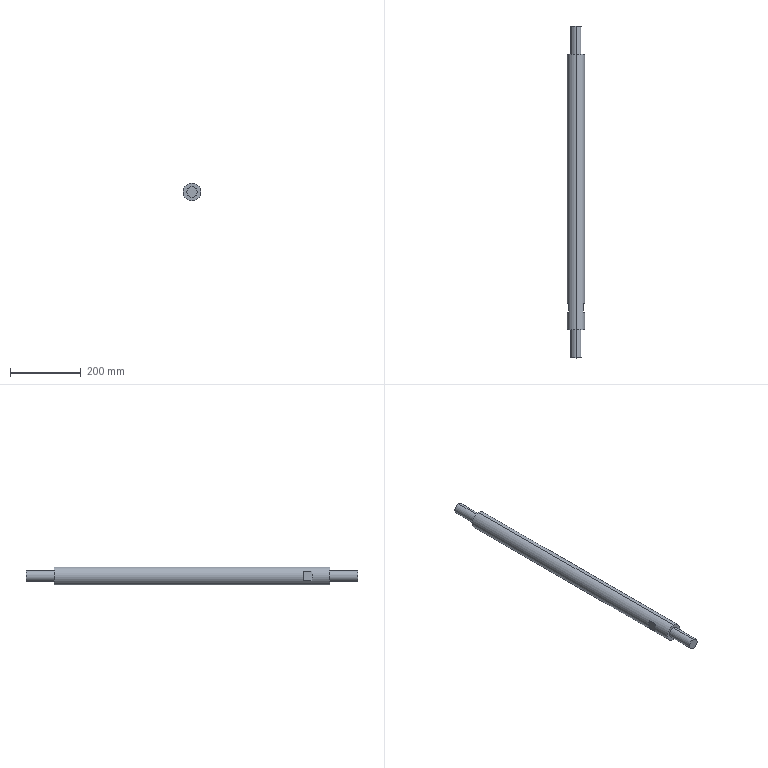Part | STEP file | 1 solid | 16 faces | box 50 x 940 x 50 mm | volume 1640944 mm3 | plane 10 | cylinder 6 | commonest cylinder face diameters 30 x4 50 x2
STEP:
#1=CARTESIAN_POINT('',(0.,0.,0.));
#2=DIRECTION('',(0.,0.,1.));
#3=DIRECTION('',(1.,0.,0.));
#4=AXIS2_PLACEMENT_3D('',#1,#2,#3);
#5=CARTESIAN_POINT('',(0.,940.,-15.));
#6=VERTEX_POINT('',#5);
#7=CARTESIAN_POINT('',(0.,940.,15.));
#8=VERTEX_POINT('',#7);
#9=CARTESIAN_POINT('',(0.,940.,0.));
#10=DIRECTION('',(0.,-1.,0.));
#11=DIRECTION('',(0.,0.,-1.));
#12=AXIS2_PLACEMENT_3D('',#9,#10,#11);
#13=CIRCLE('',#12,15.);
#14=CARTESIAN_POINT('',(0.,0.,0.));
#15=DIRECTION('',(0.,-1.,0.));
#16=DIRECTION('',(0.,0.,-1.));
#17=AXIS2_PLACEMENT_3D('',#14,#15,#16);
#18=CYLINDRICAL_SURFACE('',#17,15.);
#19=CARTESIAN_POINT('',(0.,-940.));
#20=DIRECTION('',(1.,0.));
#21=VECTOR('',#20,1.);
#22=LINE('',#19,#21);
#23=(GEOMETRIC_REPRESENTATION_CONTEXT(2)PARAMETRIC_REPRESENTATION_CONTEXT()REPRESENTATION_CONTEXT('',''));
#24=DEFINITIONAL_REPRESENTATION('',(#22),#23);
#25=PCURVE('',#18,#24);
#26=CARTESIAN_POINT('',(15.,940.,0.));
#27=DIRECTION('',(0.,1.,0.));
#28=DIRECTION('',(0.,0.,1.));
#29=AXIS2_PLACEMENT_3D('',#26,#27,#28);
#30=PLANE('',#29);
#31=CARTESIAN_POINT('',(-15.,-15.));
#32=CARTESIAN_POINT('',(-15.,10.981));
#33=CARTESIAN_POINT('',(7.5,-2.01));
#34=CARTESIAN_POINT('',(30.,-15.));
#35=CARTESIAN_POINT('',(7.5,-27.99));
#36=CARTESIAN_POINT('',(-15.,-40.981));
#37=CARTESIAN_POINT('',(-15.,-15.));
#38=(BOUNDED_CURVE()B_SPLINE_CURVE(2,(#31,#32,#33,#34,#35,#36,#37),.UNSPECIFIED.,.T.,.F.)B_SPLINE_CURVE_WITH_KNOTS((1,2,2,2,2,1),(-2.094,0.,2.094,4.189,6.283,8.378),.UNSPECIFIED.)CURVE()GEOMETRIC_REPRESENTATION_ITEM()RATIONAL_B_SPLINE_CURVE((1.,0.5,1.,0.5,1.,0.5,1.))REPRESENTATION_ITEM(''));
#39=(GEOMETRIC_REPRESENTATION_CONTEXT(2)PARAMETRIC_REPRESENTATION_CONTEXT()REPRESENTATION_CONTEXT('',''));
#40=DEFINITIONAL_REPRESENTATION('',(#38),#39);
#41=PCURVE('',#30,#40);
#42=SURFACE_CURVE('',#13,(#25,#41),.PCURVE_S1.);
#43=EDGE_CURVE('',#6,#8,#42,.T.);
#44=ORIENTED_EDGE('',*,*,#43,.T.);
#45=CARTESIAN_POINT('',(0.,860.,15.));
#46=VERTEX_POINT('',#45);
#47=CARTESIAN_POINT('',(0.,0.,15.));
#48=DIRECTION('',(0.,-1.,0.));
#49=VECTOR('',#48,1.);
#50=LINE('',#47,#49);
#51=CARTESIAN_POINT('',(3.142,0.));
#52=DIRECTION('',(0.,1.));
#53=VECTOR('',#52,1.);
#54=LINE('',#51,#53);
#55=(GEOMETRIC_REPRESENTATION_CONTEXT(2)PARAMETRIC_REPRESENTATION_CONTEXT()REPRESENTATION_CONTEXT('',''));
#56=DEFINITIONAL_REPRESENTATION('',(#54),#55);
#57=PCURVE('',#18,#56);
#58=CARTESIAN_POINT('',(0.,0.,0.));
#59=DIRECTION('',(0.,-1.,0.));
#60=DIRECTION('',(0.,0.,-1.));
#61=AXIS2_PLACEMENT_3D('',#58,#59,#60);
#62=CYLINDRICAL_SURFACE('',#61,15.);
#63=CARTESIAN_POINT('',(3.142,0.));
#64=DIRECTION('',(0.,1.));
#65=VECTOR('',#64,1.);
#66=LINE('',#63,#65);
#67=(GEOMETRIC_REPRESENTATION_CONTEXT(2)PARAMETRIC_REPRESENTATION_CONTEXT()REPRESENTATION_CONTEXT('',''));
#68=DEFINITIONAL_REPRESENTATION('',(#66),#67);
#69=PCURVE('',#62,#68);
#70=SURFACE_CURVE('',#50,(#57,#69),.PCURVE_S1.);
#71=EDGE_CURVE('',#8,#46,#70,.T.);
#72=ORIENTED_EDGE('',*,*,#71,.T.);
#73=CARTESIAN_POINT('',(0.,860.,-15.));
#74=VERTEX_POINT('',#73);
#75=CARTESIAN_POINT('',(0.,860.,0.));
#76=DIRECTION('',(0.,-1.,0.));
#77=DIRECTION('',(0.,0.,-1.));
#78=AXIS2_PLACEMENT_3D('',#75,#76,#77);
#79=CIRCLE('',#78,15.);
#80=CARTESIAN_POINT('',(0.,-860.));
#81=DIRECTION('',(1.,0.));
#82=VECTOR('',#81,1.);
#83=LINE('',#80,#82);
#84=(GEOMETRIC_REPRESENTATION_CONTEXT(2)PARAMETRIC_REPRESENTATION_CONTEXT()REPRESENTATION_CONTEXT('',''));
#85=DEFINITIONAL_REPRESENTATION('',(#83),#84);
#86=PCURVE('',#18,#85);
#87=CARTESIAN_POINT('',(25.,860.,0.));
#88=DIRECTION('',(0.,1.,0.));
#89=DIRECTION('',(0.,0.,1.));
#90=AXIS2_PLACEMENT_3D('',#87,#88,#89);
#91=PLANE('',#90);
#92=CARTESIAN_POINT('',(-15.,-25.));
#93=CARTESIAN_POINT('',(-15.,0.9808));
#94=CARTESIAN_POINT('',(7.5,-12.01));
#95=CARTESIAN_POINT('',(30.,-25.));
#96=CARTESIAN_POINT('',(7.5,-37.99));
#97=CARTESIAN_POINT('',(-15.,-50.981));
#98=CARTESIAN_POINT('',(-15.,-25.));
#99=(BOUNDED_CURVE()B_SPLINE_CURVE(2,(#92,#93,#94,#95,#96,#97,#98),.UNSPECIFIED.,.T.,.F.)B_SPLINE_CURVE_WITH_KNOTS((1,2,2,2,2,1),(-2.094,0.,2.094,4.189,6.283,8.378),.UNSPECIFIED.)CURVE()GEOMETRIC_REPRESENTATION_ITEM()RATIONAL_B_SPLINE_CURVE((1.,0.5,1.,0.5,1.,0.5,1.))REPRESENTATION_ITEM(''));
#100=(GEOMETRIC_REPRESENTATION_CONTEXT(2)PARAMETRIC_REPRESENTATION_CONTEXT()REPRESENTATION_CONTEXT('',''));
#101=DEFINITIONAL_REPRESENTATION('',(#99),#100);
#102=PCURVE('',#91,#101);
#103=SURFACE_CURVE('',#79,(#86,#102),.PCURVE_S1.);
#104=EDGE_CURVE('',#74,#46,#103,.T.);
#105=ORIENTED_EDGE('',*,*,#104,.F.);
#106=CARTESIAN_POINT('',(0.,0.,-15.));
#107=DIRECTION('',(0.,-1.,0.));
#108=VECTOR('',#107,1.);
#109=LINE('',#106,#108);
#110=CARTESIAN_POINT('',(0.,0.));
#111=DIRECTION('',(0.,1.));
#112=VECTOR('',#111,1.);
#113=LINE('',#110,#112);
#114=(GEOMETRIC_REPRESENTATION_CONTEXT(2)PARAMETRIC_REPRESENTATION_CONTEXT()REPRESENTATION_CONTEXT('',''));
#115=DEFINITIONAL_REPRESENTATION('',(#113),#114);
#116=PCURVE('',#18,#115);
#117=CARTESIAN_POINT('',(6.283,0.));
#118=DIRECTION('',(0.,1.));
#119=VECTOR('',#118,1.);
#120=LINE('',#117,#119);
#121=(GEOMETRIC_REPRESENTATION_CONTEXT(2)PARAMETRIC_REPRESENTATION_CONTEXT()REPRESENTATION_CONTEXT('',''));
#122=DEFINITIONAL_REPRESENTATION('',(#120),#121);
#123=PCURVE('',#62,#122);
#124=SURFACE_CURVE('',#109,(#116,#123),.PCURVE_S1.);
#125=EDGE_CURVE('',#6,#74,#124,.T.);
#126=ORIENTED_EDGE('',*,*,#125,.F.);
#127=EDGE_LOOP('',(#44,#72,#105,#126));
#128=FACE_BOUND('',#127,.T.);
#129=ADVANCED_FACE('',(#128),#18,.T.);
#130=CARTESIAN_POINT('',(21.,130.,-13.565));
#131=VERTEX_POINT('',#130);
#132=CARTESIAN_POINT('',(21.,155.,-13.565));
#133=VERTEX_POINT('',#132);
#134=CARTESIAN_POINT('',(21.,0.,-13.565));
#135=DIRECTION('',(0.,1.,0.));
#136=VECTOR('',#135,1.);
#137=LINE('',#134,#136);
#138=CARTESIAN_POINT('',(0.,0.,0.));
#139=DIRECTION('',(0.,-1.,0.));
#140=DIRECTION('',(0.,0.,-1.));
#141=AXIS2_PLACEMENT_3D('',#138,#139,#140);
#142=CYLINDRICAL_SURFACE('',#141,25.);
#143=CARTESIAN_POINT('',(0.9973,0.));
#144=DIRECTION('',(0.,-1.));
#145=VECTOR('',#144,1.);
#146=LINE('',#143,#145);
#147=(GEOMETRIC_REPRESENTATION_CONTEXT(2)PARAMETRIC_REPRESENTATION_CONTEXT()REPRESENTATION_CONTEXT('',''));
#148=DEFINITIONAL_REPRESENTATION('',(#146),#147);
#149=PCURVE('',#142,#148);
#150=CARTESIAN_POINT('',(21.,155.,-30.));
#151=DIRECTION('',(-1.,0.,0.));
#152=DIRECTION('',(0.,0.,1.));
#153=AXIS2_PLACEMENT_3D('',#150,#151,#152);
#154=PLANE('',#153);
#155=CARTESIAN_POINT('',(16.435,-155.));
#156=DIRECTION('',(0.,1.));
#157=VECTOR('',#156,1.);
#158=LINE('',#155,#157);
#159=(GEOMETRIC_REPRESENTATION_CONTEXT(2)PARAMETRIC_REPRESENTATION_CONTEXT()REPRESENTATION_CONTEXT('',''));
#160=DEFINITIONAL_REPRESENTATION('',(#158),#159);
#161=PCURVE('',#154,#160);
#162=SURFACE_CURVE('',#137,(#149,#161),.PCURVE_S1.);
#163=EDGE_CURVE('',#131,#133,#162,.T.);
#164=ORIENTED_EDGE('',*,*,#163,.F.);
#165=CARTESIAN_POINT('',(21.,130.,13.565));
#166=VERTEX_POINT('',#165);
#167=CARTESIAN_POINT('',(0.,130.,0.));
#168=DIRECTION('',(0.,1.,0.));
#169=DIRECTION('',(0.,0.,-1.));
#170=AXIS2_PLACEMENT_3D('',#167,#168,#169);
#171=CIRCLE('',#170,25.);
#172=CARTESIAN_POINT('',(6.283,-130.));
#173=DIRECTION('',(-1.,0.));
#174=VECTOR('',#173,1.);
#175=LINE('',#172,#174);
#176=(GEOMETRIC_REPRESENTATION_CONTEXT(2)PARAMETRIC_REPRESENTATION_CONTEXT()REPRESENTATION_CONTEXT('',''));
#177=DEFINITIONAL_REPRESENTATION('',(#175),#176);
#178=PCURVE('',#142,#177);
#179=CARTESIAN_POINT('',(65.117,130.,-30.));
#180=DIRECTION('',(0.,-1.,0.));
#181=DIRECTION('',(0.,0.,-1.));
#182=AXIS2_PLACEMENT_3D('',#179,#180,#181);
#183=PLANE('',#182);
#184=CARTESIAN_POINT('',(-5.,-65.117));
#185=CARTESIAN_POINT('',(-5.,-108.419));
#186=CARTESIAN_POINT('',(-42.5,-86.768));
#187=CARTESIAN_POINT('',(-80.,-65.117));
#188=CARTESIAN_POINT('',(-42.5,-43.467));
#189=CARTESIAN_POINT('',(-5.,-21.816));
#190=CARTESIAN_POINT('',(-5.,-65.117));
#191=(BOUNDED_CURVE()B_SPLINE_CURVE(2,(#184,#185,#186,#187,#188,#189,#190),.UNSPECIFIED.,.T.,.F.)B_SPLINE_CURVE_WITH_KNOTS((1,2,2,2,2,1),(-2.094,0.,2.094,4.189,6.283,8.378),.UNSPECIFIED.)CURVE()GEOMETRIC_REPRESENTATION_ITEM()RATIONAL_B_SPLINE_CURVE((1.,0.5,1.,0.5,1.,0.5,1.))REPRESENTATION_ITEM(''));
#192=(GEOMETRIC_REPRESENTATION_CONTEXT(2)PARAMETRIC_REPRESENTATION_CONTEXT()REPRESENTATION_CONTEXT('',''));
#193=DEFINITIONAL_REPRESENTATION('',(#191),#192);
#194=PCURVE('',#183,#193);
#195=SURFACE_CURVE('',#171,(#178,#194),.PCURVE_S1.);
#196=EDGE_CURVE('',#166,#131,#195,.T.);
#197=ORIENTED_EDGE('',*,*,#196,.F.);
#198=CARTESIAN_POINT('',(21.,155.,13.565));
#199=VERTEX_POINT('',#198);
#200=CARTESIAN_POINT('',(21.,0.,13.565));
#201=DIRECTION('',(0.,-1.,0.));
#202=VECTOR('',#201,1.);
#203=LINE('',#200,#202);
#204=CARTESIAN_POINT('',(2.144,0.));
#205=DIRECTION('',(0.,1.));
#206=VECTOR('',#205,1.);
#207=LINE('',#204,#206);
#208=(GEOMETRIC_REPRESENTATION_CONTEXT(2)PARAMETRIC_REPRESENTATION_CONTEXT()REPRESENTATION_CONTEXT('',''));
#209=DEFINITIONAL_REPRESENTATION('',(#207),#208);
#210=PCURVE('',#142,#209);
#211=CARTESIAN_POINT('',(43.565,-155.));
#212=DIRECTION('',(0.,-1.));
#213=VECTOR('',#212,1.);
#214=LINE('',#211,#213);
#215=(GEOMETRIC_REPRESENTATION_CONTEXT(2)PARAMETRIC_REPRESENTATION_CONTEXT()REPRESENTATION_CONTEXT('',''));
#216=DEFINITIONAL_REPRESENTATION('',(#214),#215);
#217=PCURVE('',#154,#216);
#218=SURFACE_CURVE('',#203,(#210,#217),.PCURVE_S1.);
#219=EDGE_CURVE('',#199,#166,#218,.T.);
#220=ORIENTED_EDGE('',*,*,#219,.F.);
#221=CARTESIAN_POINT('',(0.,155.,0.));
#222=DIRECTION('',(0.,-1.,0.));
#223=DIRECTION('',(0.,0.,1.));
#224=AXIS2_PLACEMENT_3D('',#221,#222,#223);
#225=CIRCLE('',#224,25.);
#226=CARTESIAN_POINT('',(-3.142,-155.));
#227=DIRECTION('',(1.,0.));
#228=VECTOR('',#227,1.);
#229=LINE('',#226,#228);
#230=(GEOMETRIC_REPRESENTATION_CONTEXT(2)PARAMETRIC_REPRESENTATION_CONTEXT()REPRESENTATION_CONTEXT('',''));
#231=DEFINITIONAL_REPRESENTATION('',(#229),#230);
#232=PCURVE('',#142,#231);
#233=CARTESIAN_POINT('',(65.117,155.,-30.));
#234=DIRECTION('',(0.,1.,0.));
#235=DIRECTION('',(0.,0.,1.));
#236=AXIS2_PLACEMENT_3D('',#233,#234,#235);
#237=PLANE('',#236);
#238=CARTESIAN_POINT('',(55.,-65.117));
#239=CARTESIAN_POINT('',(55.,-108.419));
#240=CARTESIAN_POINT('',(17.5,-86.768));
#241=CARTESIAN_POINT('',(-20.,-65.117));
#242=CARTESIAN_POINT('',(17.5,-43.467));
#243=CARTESIAN_POINT('',(55.,-21.816));
#244=CARTESIAN_POINT('',(55.,-65.117));
#245=(BOUNDED_CURVE()B_SPLINE_CURVE(2,(#238,#239,#240,#241,#242,#243,#244),.UNSPECIFIED.,.T.,.F.)B_SPLINE_CURVE_WITH_KNOTS((1,2,2,2,2,1),(-2.094,0.,2.094,4.189,6.283,8.378),.UNSPECIFIED.)CURVE()GEOMETRIC_REPRESENTATION_ITEM()RATIONAL_B_SPLINE_CURVE((1.,0.5,1.,0.5,1.,0.5,1.))REPRESENTATION_ITEM(''));
#246=(GEOMETRIC_REPRESENTATION_CONTEXT(2)PARAMETRIC_REPRESENTATION_CONTEXT()REPRESENTATION_CONTEXT('',''));
#247=DEFINITIONAL_REPRESENTATION('',(#245),#246);
#248=PCURVE('',#237,#247);
#249=SURFACE_CURVE('',#225,(#232,#248),.PCURVE_S1.);
#250=EDGE_CURVE('',#133,#199,#249,.T.);
#251=ORIENTED_EDGE('',*,*,#250,.F.);
#252=EDGE_LOOP('',(#164,#197,#220,#251));
#253=FACE_BOUND('',#252,.T.);
#254=CARTESIAN_POINT('',(0.,860.,-25.));
#255=VERTEX_POINT('',#254);
#256=CARTESIAN_POINT('',(0.,860.,25.));
#257=VERTEX_POINT('',#256);
#258=CARTESIAN_POINT('',(0.,860.,0.));
#259=DIRECTION('',(0.,-1.,0.));
#260=DIRECTION('',(0.,0.,-1.));
#261=AXIS2_PLACEMENT_3D('',#258,#259,#260);
#262=CIRCLE('',#261,25.);
#263=CARTESIAN_POINT('',(0.,-860.));
#264=DIRECTION('',(1.,0.));
#265=VECTOR('',#264,1.);
#266=LINE('',#263,#265);
#267=(GEOMETRIC_REPRESENTATION_CONTEXT(2)PARAMETRIC_REPRESENTATION_CONTEXT()REPRESENTATION_CONTEXT('',''));
#268=DEFINITIONAL_REPRESENTATION('',(#266),#267);
#269=PCURVE('',#142,#268);
#270=CARTESIAN_POINT('',(-25.,-25.));
#271=CARTESIAN_POINT('',(-25.,18.301));
#272=CARTESIAN_POINT('',(12.5,-3.349));
#273=CARTESIAN_POINT('',(50.,-25.));
#274=CARTESIAN_POINT('',(12.5,-46.651));
#275=CARTESIAN_POINT('',(-25.,-68.301));
#276=CARTESIAN_POINT('',(-25.,-25.));
#277=(BOUNDED_CURVE()B_SPLINE_CURVE(2,(#270,#271,#272,#273,#274,#275,#276),.UNSPECIFIED.,.T.,.F.)B_SPLINE_CURVE_WITH_KNOTS((1,2,2,2,2,1),(-2.094,0.,2.094,4.189,6.283,8.378),.UNSPECIFIED.)CURVE()GEOMETRIC_REPRESENTATION_ITEM()RATIONAL_B_SPLINE_CURVE((1.,0.5,1.,0.5,1.,0.5,1.))REPRESENTATION_ITEM(''));
#278=(GEOMETRIC_REPRESENTATION_CONTEXT(2)PARAMETRIC_REPRESENTATION_CONTEXT()REPRESENTATION_CONTEXT('',''));
#279=DEFINITIONAL_REPRESENTATION('',(#277),#278);
#280=PCURVE('',#91,#279);
#281=SURFACE_CURVE('',#262,(#269,#280),.PCURVE_S1.);
#282=EDGE_CURVE('',#255,#257,#281,.T.);
#283=ORIENTED_EDGE('',*,*,#282,.T.);
#284=CARTESIAN_POINT('',(0.,80.,25.));
#285=VERTEX_POINT('',#284);
#286=CARTESIAN_POINT('',(0.,0.,25.));
#287=DIRECTION('',(0.,-1.,0.));
#288=VECTOR('',#287,1.);
#289=LINE('',#286,#288);
#290=CARTESIAN_POINT('',(3.142,0.));
#291=DIRECTION('',(0.,1.));
#292=VECTOR('',#291,1.);
#293=LINE('',#290,#292);
#294=(GEOMETRIC_REPRESENTATION_CONTEXT(2)PARAMETRIC_REPRESENTATION_CONTEXT()REPRESENTATION_CONTEXT('',''));
#295=DEFINITIONAL_REPRESENTATION('',(#293),#294);
#296=PCURVE('',#142,#295);
#297=CARTESIAN_POINT('',(0.,0.,0.));
#298=DIRECTION('',(0.,-1.,0.));
#299=DIRECTION('',(0.,0.,-1.));
#300=AXIS2_PLACEMENT_3D('',#297,#298,#299);
#301=CYLINDRICAL_SURFACE('',#300,25.);
#302=CARTESIAN_POINT('',(3.142,0.));
#303=DIRECTION('',(0.,1.));
#304=VECTOR('',#303,1.);
#305=LINE('',#302,#304);
#306=(GEOMETRIC_REPRESENTATION_CONTEXT(2)PARAMETRIC_REPRESENTATION_CONTEXT()REPRESENTATION_CONTEXT('',''));
#307=DEFINITIONAL_REPRESENTATION('',(#305),#306);
#308=PCURVE('',#301,#307);
#309=SURFACE_CURVE('',#289,(#296,#308),.PCURVE_S1.);
#310=EDGE_CURVE('',#257,#285,#309,.T.);
#311=ORIENTED_EDGE('',*,*,#310,.T.);
#312=CARTESIAN_POINT('',(0.,80.,-25.));
#313=VERTEX_POINT('',#312);
#314=CARTESIAN_POINT('',(0.,80.,0.));
#315=DIRECTION('',(0.,-1.,0.));
#316=DIRECTION('',(0.,0.,-1.));
#317=AXIS2_PLACEMENT_3D('',#314,#315,#316);
#318=CIRCLE('',#317,25.);
#319=CARTESIAN_POINT('',(0.,-80.));
#320=DIRECTION('',(1.,0.));
#321=VECTOR('',#320,1.);
#322=LINE('',#319,#321);
#323=(GEOMETRIC_REPRESENTATION_CONTEXT(2)PARAMETRIC_REPRESENTATION_CONTEXT()REPRESENTATION_CONTEXT('',''));
#324=DEFINITIONAL_REPRESENTATION('',(#322),#323);
#325=PCURVE('',#142,#324);
#326=CARTESIAN_POINT('',(15.,80.,0.));
#327=DIRECTION('',(0.,-1.,0.));
#328=DIRECTION('',(0.,0.,-1.));
#329=AXIS2_PLACEMENT_3D('',#326,#327,#328);
#330=PLANE('',#329);
#331=CARTESIAN_POINT('',(0.,-15.));
#332=DIRECTION('',(1.,0.));
#333=AXIS2_PLACEMENT_2D('',#331,#332);
#334=CIRCLE('',#333,25.);
#335=(GEOMETRIC_REPRESENTATION_CONTEXT(2)PARAMETRIC_REPRESENTATION_CONTEXT()REPRESENTATION_CONTEXT('',''));
#336=DEFINITIONAL_REPRESENTATION('',(#334),#335);
#337=PCURVE('',#330,#336);
#338=SURFACE_CURVE('',#318,(#325,#337),.PCURVE_S1.);
#339=EDGE_CURVE('',#313,#285,#338,.T.);
#340=ORIENTED_EDGE('',*,*,#339,.F.);
#341=CARTESIAN_POINT('',(0.,0.,-25.));
#342=DIRECTION('',(0.,-1.,0.));
#343=VECTOR('',#342,1.);
#344=LINE('',#341,#343);
#345=CARTESIAN_POINT('',(0.,0.));
#346=DIRECTION('',(0.,1.));
#347=VECTOR('',#346,1.);
#348=LINE('',#345,#347);
#349=(GEOMETRIC_REPRESENTATION_CONTEXT(2)PARAMETRIC_REPRESENTATION_CONTEXT()REPRESENTATION_CONTEXT('',''));
#350=DEFINITIONAL_REPRESENTATION('',(#348),#349);
#351=PCURVE('',#142,#350);
#352=CARTESIAN_POINT('',(6.283,0.));
#353=DIRECTION('',(0.,1.));
#354=VECTOR('',#353,1.);
#355=LINE('',#352,#354);
#356=(GEOMETRIC_REPRESENTATION_CONTEXT(2)PARAMETRIC_REPRESENTATION_CONTEXT()REPRESENTATION_CONTEXT('',''));
#357=DEFINITIONAL_REPRESENTATION('',(#355),#356);
#358=PCURVE('',#301,#357);
#359=SURFACE_CURVE('',#344,(#351,#358),.PCURVE_S1.);
#360=EDGE_CURVE('',#255,#313,#359,.T.);
#361=ORIENTED_EDGE('',*,*,#360,.F.);
#362=EDGE_LOOP('',(#283,#311,#340,#361));
#363=FACE_BOUND('',#362,.T.);
#364=ADVANCED_FACE('',(#253,#363),#142,.T.);
#365=CARTESIAN_POINT('',(0.,80.,-15.));
#366=VERTEX_POINT('',#365);
#367=CARTESIAN_POINT('',(0.,80.,15.));
#368=VERTEX_POINT('',#367);
#369=CARTESIAN_POINT('',(0.,80.,0.));
#370=DIRECTION('',(0.,-1.,0.));
#371=DIRECTION('',(0.,0.,-1.));
#372=AXIS2_PLACEMENT_3D('',#369,#370,#371);
#373=CIRCLE('',#372,15.);
#374=CARTESIAN_POINT('',(0.,0.,0.));
#375=DIRECTION('',(0.,-1.,0.));
#376=DIRECTION('',(0.,0.,-1.));
#377=AXIS2_PLACEMENT_3D('',#374,#375,#376);
#378=CYLINDRICAL_SURFACE('',#377,15.);
#379=CARTESIAN_POINT('',(0.,-80.));
#380=DIRECTION('',(1.,0.));
#381=VECTOR('',#380,1.);
#382=LINE('',#379,#381);
#383=(GEOMETRIC_REPRESENTATION_CONTEXT(2)PARAMETRIC_REPRESENTATION_CONTEXT()REPRESENTATION_CONTEXT('',''));
#384=DEFINITIONAL_REPRESENTATION('',(#382),#383);
#385=PCURVE('',#378,#384);
#386=CARTESIAN_POINT('',(0.,-15.));
#387=DIRECTION('',(1.,0.));
#388=AXIS2_PLACEMENT_2D('',#386,#387);
#389=CIRCLE('',#388,15.);
#390=(GEOMETRIC_REPRESENTATION_CONTEXT(2)PARAMETRIC_REPRESENTATION_CONTEXT()REPRESENTATION_CONTEXT('',''));
#391=DEFINITIONAL_REPRESENTATION('',(#389),#390);
#392=PCURVE('',#330,#391);
#393=SURFACE_CURVE('',#373,(#385,#392),.PCURVE_S1.);
#394=EDGE_CURVE('',#366,#368,#393,.T.);
#395=ORIENTED_EDGE('',*,*,#394,.T.);
#396=CARTESIAN_POINT('',(0.,0.,15.));
#397=VERTEX_POINT('',#396);
#398=CARTESIAN_POINT('',(0.,0.,15.));
#399=DIRECTION('',(0.,-1.,0.));
#400=VECTOR('',#399,1.);
#401=LINE('',#398,#400);
#402=CARTESIAN_POINT('',(3.142,0.));
#403=DIRECTION('',(0.,1.));
#404=VECTOR('',#403,1.);
#405=LINE('',#402,#404);
#406=(GEOMETRIC_REPRESENTATION_CONTEXT(2)PARAMETRIC_REPRESENTATION_CONTEXT()REPRESENTATION_CONTEXT('',''));
#407=DEFINITIONAL_REPRESENTATION('',(#405),#406);
#408=PCURVE('',#378,#407);
#409=CARTESIAN_POINT('',(0.,0.,0.));
#410=DIRECTION('',(0.,-1.,0.));
#411=DIRECTION('',(0.,0.,-1.));
#412=AXIS2_PLACEMENT_3D('',#409,#410,#411);
#413=CYLINDRICAL_SURFACE('',#412,15.);
#414=CARTESIAN_POINT('',(3.142,0.));
#415=DIRECTION('',(0.,1.));
#416=VECTOR('',#415,1.);
#417=LINE('',#414,#416);
#418=(GEOMETRIC_REPRESENTATION_CONTEXT(2)PARAMETRIC_REPRESENTATION_CONTEXT()REPRESENTATION_CONTEXT('',''));
#419=DEFINITIONAL_REPRESENTATION('',(#417),#418);
#420=PCURVE('',#413,#419);
#421=SURFACE_CURVE('',#401,(#408,#420),.PCURVE_S1.);
#422=EDGE_CURVE('',#368,#397,#421,.T.);
#423=ORIENTED_EDGE('',*,*,#422,.T.);
#424=CARTESIAN_POINT('',(0.,0.,-15.));
#425=VERTEX_POINT('',#424);
#426=CARTESIAN_POINT('',(0.,0.,0.));
#427=DIRECTION('',(0.,-1.,0.));
#428=DIRECTION('',(0.,0.,-1.));
#429=AXIS2_PLACEMENT_3D('',#426,#427,#428);
#430=CIRCLE('',#429,15.);
#431=CARTESIAN_POINT('',(0.,0.));
#432=DIRECTION('',(1.,0.));
#433=VECTOR('',#432,1.);
#434=LINE('',#431,#433);
#435=(GEOMETRIC_REPRESENTATION_CONTEXT(2)PARAMETRIC_REPRESENTATION_CONTEXT()REPRESENTATION_CONTEXT('',''));
#436=DEFINITIONAL_REPRESENTATION('',(#434),#435);
#437=PCURVE('',#378,#436);
#438=CARTESIAN_POINT('',(0.,0.,0.));
#439=DIRECTION('',(0.,-1.,0.));
#440=DIRECTION('',(0.,0.,-1.));
#441=AXIS2_PLACEMENT_3D('',#438,#439,#440);
#442=PLANE('',#441);
#443=CARTESIAN_POINT('',(0.,0.));
#444=DIRECTION('',(1.,0.));
#445=AXIS2_PLACEMENT_2D('',#443,#444);
#446=CIRCLE('',#445,15.);
#447=(GEOMETRIC_REPRESENTATION_CONTEXT(2)PARAMETRIC_REPRESENTATION_CONTEXT()REPRESENTATION_CONTEXT('',''));
#448=DEFINITIONAL_REPRESENTATION('',(#446),#447);
#449=PCURVE('',#442,#448);
#450=SURFACE_CURVE('',#430,(#437,#449),.PCURVE_S1.);
#451=EDGE_CURVE('',#425,#397,#450,.T.);
#452=ORIENTED_EDGE('',*,*,#451,.F.);
#453=CARTESIAN_POINT('',(0.,0.,-15.));
#454=DIRECTION('',(0.,-1.,0.));
#455=VECTOR('',#454,1.);
#456=LINE('',#453,#455);
#457=CARTESIAN_POINT('',(0.,0.));
#458=DIRECTION('',(0.,1.));
#459=VECTOR('',#458,1.);
#460=LINE('',#457,#459);
#461=(GEOMETRIC_REPRESENTATION_CONTEXT(2)PARAMETRIC_REPRESENTATION_CONTEXT()REPRESENTATION_CONTEXT('',''));
#462=DEFINITIONAL_REPRESENTATION('',(#460),#461);
#463=PCURVE('',#378,#462);
#464=CARTESIAN_POINT('',(6.283,0.));
#465=DIRECTION('',(0.,1.));
#466=VECTOR('',#465,1.);
#467=LINE('',#464,#466);
#468=(GEOMETRIC_REPRESENTATION_CONTEXT(2)PARAMETRIC_REPRESENTATION_CONTEXT()REPRESENTATION_CONTEXT('',''));
#469=DEFINITIONAL_REPRESENTATION('',(#467),#468);
#470=PCURVE('',#413,#469);
#471=SURFACE_CURVE('',#456,(#463,#470),.PCURVE_S1.);
#472=EDGE_CURVE('',#366,#425,#471,.T.);
#473=ORIENTED_EDGE('',*,*,#472,.F.);
#474=EDGE_LOOP('',(#395,#423,#452,#473));
#475=FACE_BOUND('',#474,.T.);
#476=ADVANCED_FACE('',(#475),#378,.T.);
#477=ORIENTED_EDGE('',*,*,#451,.T.);
#478=CARTESIAN_POINT('',(0.,0.,0.));
#479=DIRECTION('',(0.,-1.,0.));
#480=DIRECTION('',(0.,0.,-1.));
#481=AXIS2_PLACEMENT_3D('',#478,#479,#480);
#482=CIRCLE('',#481,15.);
#483=CARTESIAN_POINT('',(0.,0.));
#484=DIRECTION('',(1.,0.));
#485=AXIS2_PLACEMENT_2D('',#483,#484);
#486=CIRCLE('',#485,15.);
#487=(GEOMETRIC_REPRESENTATION_CONTEXT(2)PARAMETRIC_REPRESENTATION_CONTEXT()REPRESENTATION_CONTEXT('',''));
#488=DEFINITIONAL_REPRESENTATION('',(#486),#487);
#489=PCURVE('',#442,#488);
#490=CARTESIAN_POINT('',(0.,0.));
#491=DIRECTION('',(1.,0.));
#492=VECTOR('',#491,1.);
#493=LINE('',#490,#492);
#494=(GEOMETRIC_REPRESENTATION_CONTEXT(2)PARAMETRIC_REPRESENTATION_CONTEXT()REPRESENTATION_CONTEXT('',''));
#495=DEFINITIONAL_REPRESENTATION('',(#493),#494);
#496=PCURVE('',#413,#495);
#497=SURFACE_CURVE('',#482,(#489,#496),.PCURVE_S1.);
#498=EDGE_CURVE('',#397,#425,#497,.T.);
#499=ORIENTED_EDGE('',*,*,#498,.T.);
#500=EDGE_LOOP('',(#477,#499));
#501=FACE_BOUND('',#500,.T.);
#502=ADVANCED_FACE('',(#501),#442,.T.);
#503=ORIENTED_EDGE('',*,*,#422,.F.);
#504=CARTESIAN_POINT('',(0.,80.,0.));
#505=DIRECTION('',(0.,-1.,0.));
#506=DIRECTION('',(0.,0.,-1.));
#507=AXIS2_PLACEMENT_3D('',#504,#505,#506);
#508=CIRCLE('',#507,15.);
#509=CARTESIAN_POINT('',(0.,-80.));
#510=DIRECTION('',(1.,0.));
#511=VECTOR('',#510,1.);
#512=LINE('',#509,#511);
#513=(GEOMETRIC_REPRESENTATION_CONTEXT(2)PARAMETRIC_REPRESENTATION_CONTEXT()REPRESENTATION_CONTEXT('',''));
#514=DEFINITIONAL_REPRESENTATION('',(#512),#513);
#515=PCURVE('',#413,#514);
#516=CARTESIAN_POINT('',(0.,-15.));
#517=DIRECTION('',(1.,0.));
#518=AXIS2_PLACEMENT_2D('',#516,#517);
#519=CIRCLE('',#518,15.);
#520=(GEOMETRIC_REPRESENTATION_CONTEXT(2)PARAMETRIC_REPRESENTATION_CONTEXT()REPRESENTATION_CONTEXT('',''));
#521=DEFINITIONAL_REPRESENTATION('',(#519),#520);
#522=PCURVE('',#330,#521);
#523=SURFACE_CURVE('',#508,(#515,#522),.PCURVE_S1.);
#524=EDGE_CURVE('',#368,#366,#523,.T.);
#525=ORIENTED_EDGE('',*,*,#524,.T.);
#526=ORIENTED_EDGE('',*,*,#472,.T.);
#527=ORIENTED_EDGE('',*,*,#498,.F.);
#528=EDGE_LOOP('',(#503,#525,#526,#527));
#529=FACE_BOUND('',#528,.T.);
#530=ADVANCED_FACE('',(#529),#413,.T.);
#531=ORIENTED_EDGE('',*,*,#339,.T.);
#532=CARTESIAN_POINT('',(0.,80.,0.));
#533=DIRECTION('',(0.,-1.,0.));
#534=DIRECTION('',(0.,0.,-1.));
#535=AXIS2_PLACEMENT_3D('',#532,#533,#534);
#536=CIRCLE('',#535,25.);
#537=CARTESIAN_POINT('',(0.,-15.));
#538=DIRECTION('',(1.,0.));
#539=AXIS2_PLACEMENT_2D('',#537,#538);
#540=CIRCLE('',#539,25.);
#541=(GEOMETRIC_REPRESENTATION_CONTEXT(2)PARAMETRIC_REPRESENTATION_CONTEXT()REPRESENTATION_CONTEXT('',''));
#542=DEFINITIONAL_REPRESENTATION('',(#540),#541);
#543=PCURVE('',#330,#542);
#544=CARTESIAN_POINT('',(0.,-80.));
#545=DIRECTION('',(1.,0.));
#546=VECTOR('',#545,1.);
#547=LINE('',#544,#546);
#548=(GEOMETRIC_REPRESENTATION_CONTEXT(2)PARAMETRIC_REPRESENTATION_CONTEXT()REPRESENTATION_CONTEXT('',''));
#549=DEFINITIONAL_REPRESENTATION('',(#547),#548);
#550=PCURVE('',#301,#549);
#551=SURFACE_CURVE('',#536,(#543,#550),.PCURVE_S1.);
#552=EDGE_CURVE('',#285,#313,#551,.T.);
#553=ORIENTED_EDGE('',*,*,#552,.T.);
#554=EDGE_LOOP('',(#531,#553));
#555=FACE_BOUND('',#554,.T.);
#556=ORIENTED_EDGE('',*,*,#394,.F.);
#557=ORIENTED_EDGE('',*,*,#524,.F.);
#558=EDGE_LOOP('',(#556,#557));
#559=FACE_BOUND('',#558,.T.);
#560=ADVANCED_FACE('',(#555,#559),#330,.T.);
#561=ORIENTED_EDGE('',*,*,#310,.F.);
#562=CARTESIAN_POINT('',(0.,860.,0.));
#563=DIRECTION('',(0.,-1.,0.));
#564=DIRECTION('',(0.,0.,-1.));
#565=AXIS2_PLACEMENT_3D('',#562,#563,#564);
#566=CIRCLE('',#565,25.);
#567=CARTESIAN_POINT('',(0.,-860.));
#568=DIRECTION('',(1.,0.));
#569=VECTOR('',#568,1.);
#570=LINE('',#567,#569);
#571=(GEOMETRIC_REPRESENTATION_CONTEXT(2)PARAMETRIC_REPRESENTATION_CONTEXT()REPRESENTATION_CONTEXT('',''));
#572=DEFINITIONAL_REPRESENTATION('',(#570),#571);
#573=PCURVE('',#301,#572);
#574=CARTESIAN_POINT('',(-25.,-25.));
#575=CARTESIAN_POINT('',(-25.,18.301));
#576=CARTESIAN_POINT('',(12.5,-3.349));
#577=CARTESIAN_POINT('',(50.,-25.));
#578=CARTESIAN_POINT('',(12.5,-46.651));
#579=CARTESIAN_POINT('',(-25.,-68.301));
#580=CARTESIAN_POINT('',(-25.,-25.));
#581=(BOUNDED_CURVE()B_SPLINE_CURVE(2,(#574,#575,#576,#577,#578,#579,#580),.UNSPECIFIED.,.T.,.F.)B_SPLINE_CURVE_WITH_KNOTS((1,2,2,2,2,1),(-2.094,0.,2.094,4.189,6.283,8.378),.UNSPECIFIED.)CURVE()GEOMETRIC_REPRESENTATION_ITEM()RATIONAL_B_SPLINE_CURVE((1.,0.5,1.,0.5,1.,0.5,1.))REPRESENTATION_ITEM(''));
#582=(GEOMETRIC_REPRESENTATION_CONTEXT(2)PARAMETRIC_REPRESENTATION_CONTEXT()REPRESENTATION_CONTEXT('',''));
#583=DEFINITIONAL_REPRESENTATION('',(#581),#582);
#584=PCURVE('',#91,#583);
#585=SURFACE_CURVE('',#566,(#573,#584),.PCURVE_S1.);
#586=EDGE_CURVE('',#257,#255,#585,.T.);
#587=ORIENTED_EDGE('',*,*,#586,.T.);
#588=ORIENTED_EDGE('',*,*,#360,.T.);
#589=ORIENTED_EDGE('',*,*,#552,.F.);
#590=EDGE_LOOP('',(#561,#587,#588,#589));
#591=FACE_BOUND('',#590,.T.);
#592=CARTESIAN_POINT('',(-21.,155.,13.565));
#593=VERTEX_POINT('',#592);
#594=CARTESIAN_POINT('',(-21.,155.,-13.565));
#595=VERTEX_POINT('',#594);
#596=CARTESIAN_POINT('',(0.,155.,0.));
#597=DIRECTION('',(0.,-1.,0.));
#598=DIRECTION('',(0.,0.,1.));
#599=AXIS2_PLACEMENT_3D('',#596,#597,#598);
#600=CIRCLE('',#599,25.);
#601=CARTESIAN_POINT('',(3.142,-155.));
#602=DIRECTION('',(1.,0.));
#603=VECTOR('',#602,1.);
#604=LINE('',#601,#603);
#605=(GEOMETRIC_REPRESENTATION_CONTEXT(2)PARAMETRIC_REPRESENTATION_CONTEXT()REPRESENTATION_CONTEXT('',''));
#606=DEFINITIONAL_REPRESENTATION('',(#604),#605);
#607=PCURVE('',#301,#606);
#608=CARTESIAN_POINT('',(-65.117,155.,-30.));
#609=DIRECTION('',(0.,1.,0.));
#610=DIRECTION('',(0.,0.,1.));
#611=AXIS2_PLACEMENT_3D('',#608,#609,#610);
#612=PLANE('',#611);
#613=CARTESIAN_POINT('',(55.,65.117));
#614=CARTESIAN_POINT('',(55.,21.816));
#615=CARTESIAN_POINT('',(17.5,43.467));
#616=CARTESIAN_POINT('',(-20.,65.117));
#617=CARTESIAN_POINT('',(17.5,86.768));
#618=CARTESIAN_POINT('',(55.,108.419));
#619=CARTESIAN_POINT('',(55.,65.117));
#620=(BOUNDED_CURVE()B_SPLINE_CURVE(2,(#613,#614,#615,#616,#617,#618,#619),.UNSPECIFIED.,.T.,.F.)B_SPLINE_CURVE_WITH_KNOTS((1,2,2,2,2,1),(-2.094,0.,2.094,4.189,6.283,8.378),.UNSPECIFIED.)CURVE()GEOMETRIC_REPRESENTATION_ITEM()RATIONAL_B_SPLINE_CURVE((1.,0.5,1.,0.5,1.,0.5,1.))REPRESENTATION_ITEM(''));
#621=(GEOMETRIC_REPRESENTATION_CONTEXT(2)PARAMETRIC_REPRESENTATION_CONTEXT()REPRESENTATION_CONTEXT('',''));
#622=DEFINITIONAL_REPRESENTATION('',(#620),#621);
#623=PCURVE('',#612,#622);
#624=SURFACE_CURVE('',#600,(#607,#623),.PCURVE_S1.);
#625=EDGE_CURVE('',#593,#595,#624,.T.);
#626=ORIENTED_EDGE('',*,*,#625,.F.);
#627=CARTESIAN_POINT('',(-21.,130.,13.565));
#628=VERTEX_POINT('',#627);
#629=CARTESIAN_POINT('',(-21.,0.,13.565));
#630=DIRECTION('',(0.,1.,0.));
#631=VECTOR('',#630,1.);
#632=LINE('',#629,#631);
#633=CARTESIAN_POINT('',(4.139,0.));
#634=DIRECTION('',(0.,-1.));
#635=VECTOR('',#634,1.);
#636=LINE('',#633,#635);
#637=(GEOMETRIC_REPRESENTATION_CONTEXT(2)PARAMETRIC_REPRESENTATION_CONTEXT()REPRESENTATION_CONTEXT('',''));
#638=DEFINITIONAL_REPRESENTATION('',(#636),#637);
#639=PCURVE('',#301,#638);
#640=CARTESIAN_POINT('',(-21.,155.,-30.));
#641=DIRECTION('',(1.,0.,0.));
#642=DIRECTION('',(0.,0.,-1.));
#643=AXIS2_PLACEMENT_3D('',#640,#641,#642);
#644=PLANE('',#643);
#645=CARTESIAN_POINT('',(-43.565,-155.));
#646=DIRECTION('',(0.,1.));
#647=VECTOR('',#646,1.);
#648=LINE('',#645,#647);
#649=(GEOMETRIC_REPRESENTATION_CONTEXT(2)PARAMETRIC_REPRESENTATION_CONTEXT()REPRESENTATION_CONTEXT('',''));
#650=DEFINITIONAL_REPRESENTATION('',(#648),#649);
#651=PCURVE('',#644,#650);
#652=SURFACE_CURVE('',#632,(#639,#651),.PCURVE_S1.);
#653=EDGE_CURVE('',#628,#593,#652,.T.);
#654=ORIENTED_EDGE('',*,*,#653,.F.);
#655=CARTESIAN_POINT('',(-21.,130.,-13.565));
#656=VERTEX_POINT('',#655);
#657=CARTESIAN_POINT('',(0.,130.,0.));
#658=DIRECTION('',(0.,1.,0.));
#659=DIRECTION('',(0.,0.,-1.));
#660=AXIS2_PLACEMENT_3D('',#657,#658,#659);
#661=CIRCLE('',#660,25.);
#662=CARTESIAN_POINT('',(6.283,-130.));
#663=DIRECTION('',(-1.,0.));
#664=VECTOR('',#663,1.);
#665=LINE('',#662,#664);
#666=(GEOMETRIC_REPRESENTATION_CONTEXT(2)PARAMETRIC_REPRESENTATION_CONTEXT()REPRESENTATION_CONTEXT('',''));
#667=DEFINITIONAL_REPRESENTATION('',(#665),#666);
#668=PCURVE('',#301,#667);
#669=CARTESIAN_POINT('',(-65.117,130.,-30.));
#670=DIRECTION('',(0.,-1.,0.));
#671=DIRECTION('',(0.,0.,-1.));
#672=AXIS2_PLACEMENT_3D('',#669,#670,#671);
#673=PLANE('',#672);
#674=CARTESIAN_POINT('',(-5.,65.117));
#675=CARTESIAN_POINT('',(-5.,21.816));
#676=CARTESIAN_POINT('',(-42.5,43.467));
#677=CARTESIAN_POINT('',(-80.,65.117));
#678=CARTESIAN_POINT('',(-42.5,86.768));
#679=CARTESIAN_POINT('',(-5.,108.419));
#680=CARTESIAN_POINT('',(-5.,65.117));
#681=(BOUNDED_CURVE()B_SPLINE_CURVE(2,(#674,#675,#676,#677,#678,#679,#680),.UNSPECIFIED.,.T.,.F.)B_SPLINE_CURVE_WITH_KNOTS((1,2,2,2,2,1),(-2.094,0.,2.094,4.189,6.283,8.378),.UNSPECIFIED.)CURVE()GEOMETRIC_REPRESENTATION_ITEM()RATIONAL_B_SPLINE_CURVE((1.,0.5,1.,0.5,1.,0.5,1.))REPRESENTATION_ITEM(''));
#682=(GEOMETRIC_REPRESENTATION_CONTEXT(2)PARAMETRIC_REPRESENTATION_CONTEXT()REPRESENTATION_CONTEXT('',''));
#683=DEFINITIONAL_REPRESENTATION('',(#681),#682);
#684=PCURVE('',#673,#683);
#685=SURFACE_CURVE('',#661,(#668,#684),.PCURVE_S1.);
#686=EDGE_CURVE('',#656,#628,#685,.T.);
#687=ORIENTED_EDGE('',*,*,#686,.F.);
#688=CARTESIAN_POINT('',(-21.,0.,-13.565));
#689=DIRECTION('',(0.,-1.,0.));
#690=VECTOR('',#689,1.);
#691=LINE('',#688,#690);
#692=CARTESIAN_POINT('',(5.286,0.));
#693=DIRECTION('',(0.,1.));
#694=VECTOR('',#693,1.);
#695=LINE('',#692,#694);
#696=(GEOMETRIC_REPRESENTATION_CONTEXT(2)PARAMETRIC_REPRESENTATION_CONTEXT()REPRESENTATION_CONTEXT('',''));
#697=DEFINITIONAL_REPRESENTATION('',(#695),#696);
#698=PCURVE('',#301,#697);
#699=CARTESIAN_POINT('',(-16.435,-155.));
#700=DIRECTION('',(0.,-1.));
#701=VECTOR('',#700,1.);
#702=LINE('',#699,#701);
#703=(GEOMETRIC_REPRESENTATION_CONTEXT(2)PARAMETRIC_REPRESENTATION_CONTEXT()REPRESENTATION_CONTEXT('',''));
#704=DEFINITIONAL_REPRESENTATION('',(#702),#703);
#705=PCURVE('',#644,#704);
#706=SURFACE_CURVE('',#691,(#698,#705),.PCURVE_S1.);
#707=EDGE_CURVE('',#595,#656,#706,.T.);
#708=ORIENTED_EDGE('',*,*,#707,.F.);
#709=EDGE_LOOP('',(#626,#654,#687,#708));
#710=FACE_BOUND('',#709,.T.);
#711=ADVANCED_FACE('',(#591,#710),#301,.T.);
#712=ORIENTED_EDGE('',*,*,#104,.T.);
#713=CARTESIAN_POINT('',(0.,860.,0.));
#714=DIRECTION('',(0.,-1.,0.));
#715=DIRECTION('',(0.,0.,-1.));
#716=AXIS2_PLACEMENT_3D('',#713,#714,#715);
#717=CIRCLE('',#716,15.);
#718=CARTESIAN_POINT('',(-15.,-25.));
#719=CARTESIAN_POINT('',(-15.,0.9808));
#720=CARTESIAN_POINT('',(7.5,-12.01));
#721=CARTESIAN_POINT('',(30.,-25.));
#722=CARTESIAN_POINT('',(7.5,-37.99));
#723=CARTESIAN_POINT('',(-15.,-50.981));
#724=CARTESIAN_POINT('',(-15.,-25.));
#725=(BOUNDED_CURVE()B_SPLINE_CURVE(2,(#718,#719,#720,#721,#722,#723,#724),.UNSPECIFIED.,.T.,.F.)B_SPLINE_CURVE_WITH_KNOTS((1,2,2,2,2,1),(-2.094,0.,2.094,4.189,6.283,8.378),.UNSPECIFIED.)CURVE()GEOMETRIC_REPRESENTATION_ITEM()RATIONAL_B_SPLINE_CURVE((1.,0.5,1.,0.5,1.,0.5,1.))REPRESENTATION_ITEM(''));
#726=(GEOMETRIC_REPRESENTATION_CONTEXT(2)PARAMETRIC_REPRESENTATION_CONTEXT()REPRESENTATION_CONTEXT('',''));
#727=DEFINITIONAL_REPRESENTATION('',(#725),#726);
#728=PCURVE('',#91,#727);
#729=CARTESIAN_POINT('',(0.,-860.));
#730=DIRECTION('',(1.,0.));
#731=VECTOR('',#730,1.);
#732=LINE('',#729,#731);
#733=(GEOMETRIC_REPRESENTATION_CONTEXT(2)PARAMETRIC_REPRESENTATION_CONTEXT()REPRESENTATION_CONTEXT('',''));
#734=DEFINITIONAL_REPRESENTATION('',(#732),#733);
#735=PCURVE('',#62,#734);
#736=SURFACE_CURVE('',#717,(#728,#735),.PCURVE_S1.);
#737=EDGE_CURVE('',#46,#74,#736,.T.);
#738=ORIENTED_EDGE('',*,*,#737,.T.);
#739=EDGE_LOOP('',(#712,#738));
#740=FACE_BOUND('',#739,.T.);
#741=ORIENTED_EDGE('',*,*,#282,.F.);
#742=ORIENTED_EDGE('',*,*,#586,.F.);
#743=EDGE_LOOP('',(#741,#742));
#744=FACE_BOUND('',#743,.T.);
#745=ADVANCED_FACE('',(#740,#744),#91,.T.);
#746=ORIENTED_EDGE('',*,*,#71,.F.);
#747=CARTESIAN_POINT('',(0.,940.,0.));
#748=DIRECTION('',(0.,-1.,0.));
#749=DIRECTION('',(0.,0.,-1.));
#750=AXIS2_PLACEMENT_3D('',#747,#748,#749);
#751=CIRCLE('',#750,15.);
#752=CARTESIAN_POINT('',(0.,-940.));
#753=DIRECTION('',(1.,0.));
#754=VECTOR('',#753,1.);
#755=LINE('',#752,#754);
#756=(GEOMETRIC_REPRESENTATION_CONTEXT(2)PARAMETRIC_REPRESENTATION_CONTEXT()REPRESENTATION_CONTEXT('',''));
#757=DEFINITIONAL_REPRESENTATION('',(#755),#756);
#758=PCURVE('',#62,#757);
#759=CARTESIAN_POINT('',(-15.,-15.));
#760=CARTESIAN_POINT('',(-15.,10.981));
#761=CARTESIAN_POINT('',(7.5,-2.01));
#762=CARTESIAN_POINT('',(30.,-15.));
#763=CARTESIAN_POINT('',(7.5,-27.99));
#764=CARTESIAN_POINT('',(-15.,-40.981));
#765=CARTESIAN_POINT('',(-15.,-15.));
#766=(BOUNDED_CURVE()B_SPLINE_CURVE(2,(#759,#760,#761,#762,#763,#764,#765),.UNSPECIFIED.,.T.,.F.)B_SPLINE_CURVE_WITH_KNOTS((1,2,2,2,2,1),(-2.094,0.,2.094,4.189,6.283,8.378),.UNSPECIFIED.)CURVE()GEOMETRIC_REPRESENTATION_ITEM()RATIONAL_B_SPLINE_CURVE((1.,0.5,1.,0.5,1.,0.5,1.))REPRESENTATION_ITEM(''));
#767=(GEOMETRIC_REPRESENTATION_CONTEXT(2)PARAMETRIC_REPRESENTATION_CONTEXT()REPRESENTATION_CONTEXT('',''));
#768=DEFINITIONAL_REPRESENTATION('',(#766),#767);
#769=PCURVE('',#30,#768);
#770=SURFACE_CURVE('',#751,(#758,#769),.PCURVE_S1.);
#771=EDGE_CURVE('',#8,#6,#770,.T.);
#772=ORIENTED_EDGE('',*,*,#771,.T.);
#773=ORIENTED_EDGE('',*,*,#125,.T.);
#774=ORIENTED_EDGE('',*,*,#737,.F.);
#775=EDGE_LOOP('',(#746,#772,#773,#774));
#776=FACE_BOUND('',#775,.T.);
#777=ADVANCED_FACE('',(#776),#62,.T.);
#778=ORIENTED_EDGE('',*,*,#43,.F.);
#779=ORIENTED_EDGE('',*,*,#771,.F.);
#780=EDGE_LOOP('',(#778,#779));
#781=FACE_BOUND('',#780,.T.);
#782=ADVANCED_FACE('',(#781),#30,.T.);
#783=ORIENTED_EDGE('',*,*,#625,.T.);
#784=CARTESIAN_POINT('',(-21.,155.,-30.));
#785=DIRECTION('',(0.,0.,1.));
#786=VECTOR('',#785,1.);
#787=LINE('',#784,#786);
#788=CARTESIAN_POINT('',(0.,44.117));
#789=DIRECTION('',(1.,0.));
#790=VECTOR('',#789,1.);
#791=LINE('',#788,#790);
#792=(GEOMETRIC_REPRESENTATION_CONTEXT(2)PARAMETRIC_REPRESENTATION_CONTEXT()REPRESENTATION_CONTEXT('',''));
#793=DEFINITIONAL_REPRESENTATION('',(#791),#792);
#794=PCURVE('',#612,#793);
#795=CARTESIAN_POINT('',(0.,0.));
#796=DIRECTION('',(-1.,0.));
#797=VECTOR('',#796,1.);
#798=LINE('',#795,#797);
#799=(GEOMETRIC_REPRESENTATION_CONTEXT(2)PARAMETRIC_REPRESENTATION_CONTEXT()REPRESENTATION_CONTEXT('',''));
#800=DEFINITIONAL_REPRESENTATION('',(#798),#799);
#801=PCURVE('',#644,#800);
#802=SURFACE_CURVE('',#787,(#794,#801),.PCURVE_S1.);
#803=EDGE_CURVE('',#595,#593,#802,.T.);
#804=ORIENTED_EDGE('',*,*,#803,.T.);
#805=EDGE_LOOP('',(#783,#804));
#806=FACE_BOUND('',#805,.T.);
#807=ADVANCED_FACE('',(#806),#612,.F.);
#808=ORIENTED_EDGE('',*,*,#653,.T.);
#809=ORIENTED_EDGE('',*,*,#803,.F.);
#810=ORIENTED_EDGE('',*,*,#707,.T.);
#811=CARTESIAN_POINT('',(-21.,130.,-30.));
#812=DIRECTION('',(0.,0.,1.));
#813=VECTOR('',#812,1.);
#814=LINE('',#811,#813);
#815=CARTESIAN_POINT('',(0.,-25.));
#816=DIRECTION('',(-1.,0.));
#817=VECTOR('',#816,1.);
#818=LINE('',#815,#817);
#819=(GEOMETRIC_REPRESENTATION_CONTEXT(2)PARAMETRIC_REPRESENTATION_CONTEXT()REPRESENTATION_CONTEXT('',''));
#820=DEFINITIONAL_REPRESENTATION('',(#818),#819);
#821=PCURVE('',#644,#820);
#822=CARTESIAN_POINT('',(0.,44.117));
#823=DIRECTION('',(-1.,0.));
#824=VECTOR('',#823,1.);
#825=LINE('',#822,#824);
#826=(GEOMETRIC_REPRESENTATION_CONTEXT(2)PARAMETRIC_REPRESENTATION_CONTEXT()REPRESENTATION_CONTEXT('',''));
#827=DEFINITIONAL_REPRESENTATION('',(#825),#826);
#828=PCURVE('',#673,#827);
#829=SURFACE_CURVE('',#814,(#821,#828),.PCURVE_S1.);
#830=EDGE_CURVE('',#656,#628,#829,.T.);
#831=ORIENTED_EDGE('',*,*,#830,.T.);
#832=EDGE_LOOP('',(#808,#809,#810,#831));
#833=FACE_BOUND('',#832,.T.);
#834=ADVANCED_FACE('',(#833),#644,.F.);
#835=ORIENTED_EDGE('',*,*,#686,.T.);
#836=ORIENTED_EDGE('',*,*,#830,.F.);
#837=EDGE_LOOP('',(#835,#836));
#838=FACE_BOUND('',#837,.T.);
#839=ADVANCED_FACE('',(#838),#673,.F.);
#840=ORIENTED_EDGE('',*,*,#250,.T.);
#841=CARTESIAN_POINT('',(21.,155.,-30.));
#842=DIRECTION('',(0.,0.,1.));
#843=VECTOR('',#842,1.);
#844=LINE('',#841,#843);
#845=CARTESIAN_POINT('',(0.,-44.117));
#846=DIRECTION('',(1.,0.));
#847=VECTOR('',#846,1.);
#848=LINE('',#845,#847);
#849=(GEOMETRIC_REPRESENTATION_CONTEXT(2)PARAMETRIC_REPRESENTATION_CONTEXT()REPRESENTATION_CONTEXT('',''));
#850=DEFINITIONAL_REPRESENTATION('',(#848),#849);
#851=PCURVE('',#237,#850);
#852=CARTESIAN_POINT('',(0.,0.));
#853=DIRECTION('',(1.,0.));
#854=VECTOR('',#853,1.);
#855=LINE('',#852,#854);
#856=(GEOMETRIC_REPRESENTATION_CONTEXT(2)PARAMETRIC_REPRESENTATION_CONTEXT()REPRESENTATION_CONTEXT('',''));
#857=DEFINITIONAL_REPRESENTATION('',(#855),#856);
#858=PCURVE('',#154,#857);
#859=SURFACE_CURVE('',#844,(#851,#858),.PCURVE_S1.);
#860=EDGE_CURVE('',#133,#199,#859,.T.);
#861=ORIENTED_EDGE('',*,*,#860,.F.);
#862=EDGE_LOOP('',(#840,#861));
#863=FACE_BOUND('',#862,.T.);
#864=ADVANCED_FACE('',(#863),#237,.F.);
#865=ORIENTED_EDGE('',*,*,#196,.T.);
#866=CARTESIAN_POINT('',(21.,130.,-30.));
#867=DIRECTION('',(0.,0.,1.));
#868=VECTOR('',#867,1.);
#869=LINE('',#866,#868);
#870=CARTESIAN_POINT('',(0.,-44.117));
#871=DIRECTION('',(-1.,0.));
#872=VECTOR('',#871,1.);
#873=LINE('',#870,#872);
#874=(GEOMETRIC_REPRESENTATION_CONTEXT(2)PARAMETRIC_REPRESENTATION_CONTEXT()REPRESENTATION_CONTEXT('',''));
#875=DEFINITIONAL_REPRESENTATION('',(#873),#874);
#876=PCURVE('',#183,#875);
#877=CARTESIAN_POINT('',(0.,-25.));
#878=DIRECTION('',(1.,0.));
#879=VECTOR('',#878,1.);
#880=LINE('',#877,#879);
#881=(GEOMETRIC_REPRESENTATION_CONTEXT(2)PARAMETRIC_REPRESENTATION_CONTEXT()REPRESENTATION_CONTEXT('',''));
#882=DEFINITIONAL_REPRESENTATION('',(#880),#881);
#883=PCURVE('',#154,#882);
#884=SURFACE_CURVE('',#869,(#876,#883),.PCURVE_S1.);
#885=EDGE_CURVE('',#131,#166,#884,.T.);
#886=ORIENTED_EDGE('',*,*,#885,.T.);
#887=EDGE_LOOP('',(#865,#886));
#888=FACE_BOUND('',#887,.T.);
#889=ADVANCED_FACE('',(#888),#183,.F.);
#890=ORIENTED_EDGE('',*,*,#163,.T.);
#891=ORIENTED_EDGE('',*,*,#860,.T.);
#892=ORIENTED_EDGE('',*,*,#219,.T.);
#893=ORIENTED_EDGE('',*,*,#885,.F.);
#894=EDGE_LOOP('',(#890,#891,#892,#893));
#895=FACE_BOUND('',#894,.T.);
#896=ADVANCED_FACE('',(#895),#154,.F.);
#897=CLOSED_SHELL('',(#129,#364,#476,#502,#530,#560,#711,#745,#777,#782,#807,#834,#839,#864,#889,#896));
#898=MANIFOLD_SOLID_BREP('',#897);
#899=(LENGTH_UNIT()NAMED_UNIT(*)SI_UNIT(.MILLI.,.METRE.));
#900=UNCERTAINTY_MEASURE_WITH_UNIT(LENGTH_MEASURE(0.0000001),#899,'','');
#901=(NAMED_UNIT(*)PLANE_ANGLE_UNIT()SI_UNIT($,.RADIAN.));
#902=(NAMED_UNIT(*)SI_UNIT($,.STERADIAN.)SOLID_ANGLE_UNIT());
#903=(GEOMETRIC_REPRESENTATION_CONTEXT(3)GLOBAL_UNCERTAINTY_ASSIGNED_CONTEXT((#900))GLOBAL_UNIT_ASSIGNED_CONTEXT((#899,#901,#902))REPRESENTATION_CONTEXT('',''));
#904=ADVANCED_BREP_SHAPE_REPRESENTATION('',(#4,#898),#903);